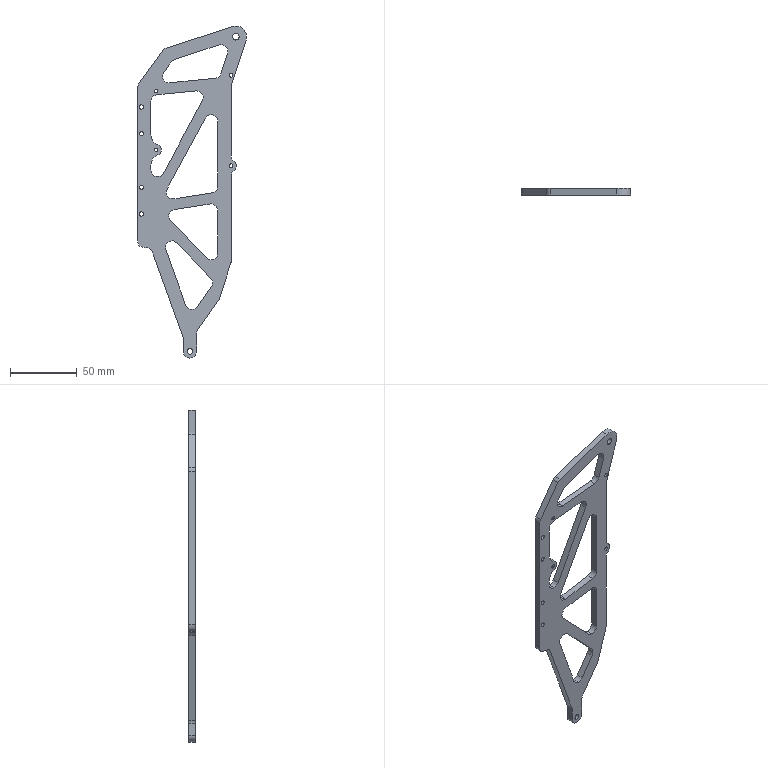Part | SolidWorks | features Fillet 3, ICE 3, Chamfer 1, Extrusion 1 | 1 solid | 93 faces | box 81.5 x 5 x 248 mm | volume 38824 mm3 | cylinder 62 | plane 31 | commonest cylinder face diameters 10 x37 2.7 x8 3.2 x8 16 x3 4.2 x2 5 x2